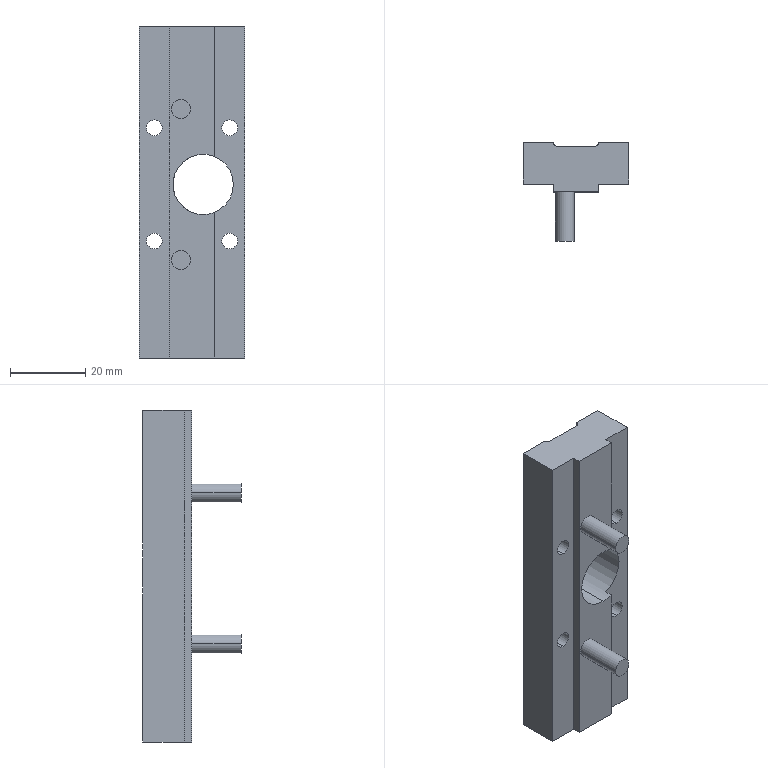Part | SolidWorks | features BaseBody 1 | 1 solid | 33 faces | box 28 x 26.1 x 88 mm | volume 25740 mm3 | cylinder 17 | plane 16 | commonest cylinder face diameters 4.2 x8 5 x4 2 x3 16 x2
STEP:
#1=CARTESIAN_POINT('',(-10.,2.,28.9));
#2=VERTEX_POINT('',#1);
#3=CARTESIAN_POINT('',(-10.,2.,33.1));
#4=VERTEX_POINT('',#3);
#5=CARTESIAN_POINT('',(-10.,2.,31.));
#6=DIRECTION('',(0.,1.,0.));
#7=DIRECTION('',(0.,0.,1.));
#8=AXIS2_PLACEMENT_3D('',#5,#6,#7);
#9=CIRCLE('',#8,2.1);
#10=EDGE_CURVE('',#2,#4,#9,.T.);
#11=ORIENTED_EDGE('',*,*,#10,.F.);
#12=CARTESIAN_POINT('',(-10.,13.,28.9));
#13=VERTEX_POINT('',#12);
#14=CARTESIAN_POINT('',(-10.,13.,28.9));
#15=DIRECTION('',(0.,1.,0.));
#16=VECTOR('',#15,1000.);
#17=LINE('',#14,#16);
#18=EDGE_CURVE('',#2,#13,#17,.T.);
#19=ORIENTED_EDGE('',*,*,#18,.T.);
#20=CARTESIAN_POINT('',(-10.,13.,33.1));
#21=VERTEX_POINT('',#20);
#22=CARTESIAN_POINT('',(-10.,13.,31.));
#23=DIRECTION('',(0.,1.,0.));
#24=DIRECTION('',(0.,0.,1.));
#25=AXIS2_PLACEMENT_3D('',#22,#23,#24);
#26=CIRCLE('',#25,2.1);
#27=EDGE_CURVE('',#13,#21,#26,.T.);
#28=ORIENTED_EDGE('',*,*,#27,.T.);
#29=CARTESIAN_POINT('',(-10.,13.,33.1));
#30=DIRECTION('',(0.,1.,0.));
#31=VECTOR('',#30,1000.);
#32=LINE('',#29,#31);
#33=EDGE_CURVE('',#4,#21,#32,.T.);
#34=ORIENTED_EDGE('',*,*,#33,.F.);
#35=EDGE_LOOP('',(#11,#19,#28,#34));
#36=FACE_OUTER_BOUND('',#35,.T.);
#37=CARTESIAN_POINT('',(-10.,13.,31.));
#38=DIRECTION('',(0.,1.,0.));
#39=DIRECTION('',(0.,0.,1.));
#40=AXIS2_PLACEMENT_3D('',#37,#38,#39);
#41=CYLINDRICAL_SURFACE('',#40,2.1);
#42=ADVANCED_FACE('',(#36),#41,.F.);
#43=CARTESIAN_POINT('',(-10.,2.,58.9));
#44=VERTEX_POINT('',#43);
#45=CARTESIAN_POINT('',(-10.,2.,63.1));
#46=VERTEX_POINT('',#45);
#47=CARTESIAN_POINT('',(-10.,2.,61.));
#48=DIRECTION('',(0.,1.,0.));
#49=DIRECTION('',(0.,0.,1.));
#50=AXIS2_PLACEMENT_3D('',#47,#48,#49);
#51=CIRCLE('',#50,2.1);
#52=EDGE_CURVE('',#44,#46,#51,.T.);
#53=ORIENTED_EDGE('',*,*,#52,.F.);
#54=CARTESIAN_POINT('',(-10.,13.,58.9));
#55=VERTEX_POINT('',#54);
#56=CARTESIAN_POINT('',(-10.,13.,58.9));
#57=DIRECTION('',(0.,1.,0.));
#58=VECTOR('',#57,1000.);
#59=LINE('',#56,#58);
#60=EDGE_CURVE('',#44,#55,#59,.T.);
#61=ORIENTED_EDGE('',*,*,#60,.T.);
#62=CARTESIAN_POINT('',(-10.,13.,63.1));
#63=VERTEX_POINT('',#62);
#64=CARTESIAN_POINT('',(-10.,13.,61.));
#65=DIRECTION('',(0.,1.,0.));
#66=DIRECTION('',(0.,0.,1.));
#67=AXIS2_PLACEMENT_3D('',#64,#65,#66);
#68=CIRCLE('',#67,2.1);
#69=EDGE_CURVE('',#55,#63,#68,.T.);
#70=ORIENTED_EDGE('',*,*,#69,.T.);
#71=CARTESIAN_POINT('',(-10.,13.,63.1));
#72=DIRECTION('',(0.,1.,0.));
#73=VECTOR('',#72,1000.);
#74=LINE('',#71,#73);
#75=EDGE_CURVE('',#46,#63,#74,.T.);
#76=ORIENTED_EDGE('',*,*,#75,.F.);
#77=EDGE_LOOP('',(#53,#61,#70,#76));
#78=FACE_OUTER_BOUND('',#77,.T.);
#79=CARTESIAN_POINT('',(-10.,13.,61.));
#80=DIRECTION('',(0.,1.,0.));
#81=DIRECTION('',(0.,0.,1.));
#82=AXIS2_PLACEMENT_3D('',#79,#80,#81);
#83=CYLINDRICAL_SURFACE('',#82,2.1);
#84=ADVANCED_FACE('',(#78),#83,.F.);
#85=CARTESIAN_POINT('',(10.,2.,28.9));
#86=VERTEX_POINT('',#85);
#87=CARTESIAN_POINT('',(10.,2.,33.1));
#88=VERTEX_POINT('',#87);
#89=CARTESIAN_POINT('',(10.,2.,31.));
#90=DIRECTION('',(0.,1.,0.));
#91=DIRECTION('',(-1.,0.,0.));
#92=AXIS2_PLACEMENT_3D('',#89,#90,#91);
#93=CIRCLE('',#92,2.1);
#94=EDGE_CURVE('',#86,#88,#93,.T.);
#95=ORIENTED_EDGE('',*,*,#94,.F.);
#96=CARTESIAN_POINT('',(10.,13.,28.9));
#97=VERTEX_POINT('',#96);
#98=CARTESIAN_POINT('',(10.,13.,28.9));
#99=DIRECTION('',(0.,1.,0.));
#100=VECTOR('',#99,1000.);
#101=LINE('',#98,#100);
#102=EDGE_CURVE('',#86,#97,#101,.T.);
#103=ORIENTED_EDGE('',*,*,#102,.T.);
#104=CARTESIAN_POINT('',(10.,13.,33.1));
#105=VERTEX_POINT('',#104);
#106=CARTESIAN_POINT('',(10.,13.,31.));
#107=DIRECTION('',(0.,1.,0.));
#108=DIRECTION('',(0.,0.,1.));
#109=AXIS2_PLACEMENT_3D('',#106,#107,#108);
#110=CIRCLE('',#109,2.1);
#111=EDGE_CURVE('',#97,#105,#110,.T.);
#112=ORIENTED_EDGE('',*,*,#111,.T.);
#113=CARTESIAN_POINT('',(10.,13.,33.1));
#114=DIRECTION('',(0.,1.,0.));
#115=VECTOR('',#114,1000.);
#116=LINE('',#113,#115);
#117=EDGE_CURVE('',#88,#105,#116,.T.);
#118=ORIENTED_EDGE('',*,*,#117,.F.);
#119=EDGE_LOOP('',(#95,#103,#112,#118));
#120=FACE_OUTER_BOUND('',#119,.T.);
#121=CARTESIAN_POINT('',(10.,13.,31.));
#122=DIRECTION('',(0.,1.,0.));
#123=DIRECTION('',(0.,0.,1.));
#124=AXIS2_PLACEMENT_3D('',#121,#122,#123);
#125=CYLINDRICAL_SURFACE('',#124,2.1);
#126=ADVANCED_FACE('',(#120),#125,.F.);
#127=CARTESIAN_POINT('',(10.,2.,58.9));
#128=VERTEX_POINT('',#127);
#129=CARTESIAN_POINT('',(10.,2.,63.1));
#130=VERTEX_POINT('',#129);
#131=CARTESIAN_POINT('',(10.,2.,61.));
#132=DIRECTION('',(0.,1.,0.));
#133=DIRECTION('',(-1.,0.,0.));
#134=AXIS2_PLACEMENT_3D('',#131,#132,#133);
#135=CIRCLE('',#134,2.1);
#136=EDGE_CURVE('',#128,#130,#135,.T.);
#137=ORIENTED_EDGE('',*,*,#136,.F.);
#138=CARTESIAN_POINT('',(10.,13.,58.9));
#139=VERTEX_POINT('',#138);
#140=CARTESIAN_POINT('',(10.,13.,58.9));
#141=DIRECTION('',(0.,1.,0.));
#142=VECTOR('',#141,1000.);
#143=LINE('',#140,#142);
#144=EDGE_CURVE('',#128,#139,#143,.T.);
#145=ORIENTED_EDGE('',*,*,#144,.T.);
#146=CARTESIAN_POINT('',(10.,13.,63.1));
#147=VERTEX_POINT('',#146);
#148=CARTESIAN_POINT('',(10.,13.,61.));
#149=DIRECTION('',(0.,1.,0.));
#150=DIRECTION('',(0.,0.,1.));
#151=AXIS2_PLACEMENT_3D('',#148,#149,#150);
#152=CIRCLE('',#151,2.1);
#153=EDGE_CURVE('',#139,#147,#152,.T.);
#154=ORIENTED_EDGE('',*,*,#153,.T.);
#155=CARTESIAN_POINT('',(10.,13.,63.1));
#156=DIRECTION('',(0.,1.,0.));
#157=VECTOR('',#156,1000.);
#158=LINE('',#155,#157);
#159=EDGE_CURVE('',#130,#147,#158,.T.);
#160=ORIENTED_EDGE('',*,*,#159,.F.);
#161=EDGE_LOOP('',(#137,#145,#154,#160));
#162=FACE_OUTER_BOUND('',#161,.T.);
#163=CARTESIAN_POINT('',(10.,13.,61.));
#164=DIRECTION('',(0.,1.,0.));
#165=DIRECTION('',(0.,0.,1.));
#166=AXIS2_PLACEMENT_3D('',#163,#164,#165);
#167=CYLINDRICAL_SURFACE('',#166,2.1);
#168=ADVANCED_FACE('',(#162),#167,.F.);
#169=CARTESIAN_POINT('',(2.95,12.,54.));
#170=VERTEX_POINT('',#169);
#171=CARTESIAN_POINT('',(-5.,12.,46.893));
#172=VERTEX_POINT('',#171);
#173=CARTESIAN_POINT('',(2.95,12.,46.));
#174=DIRECTION('',(0.,-1.,0.));
#175=DIRECTION('',(1.,0.,0.));
#176=AXIS2_PLACEMENT_3D('',#173,#174,#175);
#177=CIRCLE('',#176,8.);
#178=EDGE_CURVE('',#170,#172,#177,.T.);
#179=ORIENTED_EDGE('',*,*,#178,.F.);
#180=CARTESIAN_POINT('',(2.95,0.,54.));
#181=VERTEX_POINT('',#180);
#182=CARTESIAN_POINT('',(2.95,0.,54.));
#183=DIRECTION('',(0.,-1.,0.));
#184=VECTOR('',#183,1000.);
#185=LINE('',#182,#184);
#186=EDGE_CURVE('',#170,#181,#185,.T.);
#187=ORIENTED_EDGE('',*,*,#186,.T.);
#188=CARTESIAN_POINT('',(2.95,0.,38.));
#189=VERTEX_POINT('',#188);
#190=CARTESIAN_POINT('',(2.95,0.,46.));
#191=DIRECTION('',(0.,-1.,0.));
#192=DIRECTION('',(0.,0.,-1.));
#193=AXIS2_PLACEMENT_3D('',#190,#191,#192);
#194=CIRCLE('',#193,8.);
#195=EDGE_CURVE('',#181,#189,#194,.T.);
#196=ORIENTED_EDGE('',*,*,#195,.T.);
#197=CARTESIAN_POINT('',(2.95,12.,38.));
#198=VERTEX_POINT('',#197);
#199=CARTESIAN_POINT('',(2.95,0.,38.));
#200=DIRECTION('',(0.,-1.,0.));
#201=VECTOR('',#200,1000.);
#202=LINE('',#199,#201);
#203=EDGE_CURVE('',#198,#189,#202,.T.);
#204=ORIENTED_EDGE('',*,*,#203,.F.);
#205=CARTESIAN_POINT('',(-5.,12.,45.107));
#206=VERTEX_POINT('',#205);
#207=CARTESIAN_POINT('',(2.95,12.,46.));
#208=DIRECTION('',(0.,-1.,0.));
#209=DIRECTION('',(1.,0.,0.));
#210=AXIS2_PLACEMENT_3D('',#207,#208,#209);
#211=CIRCLE('',#210,8.);
#212=EDGE_CURVE('',#206,#198,#211,.T.);
#213=ORIENTED_EDGE('',*,*,#212,.F.);
#214=CARTESIAN_POINT('',(-5.,12.,46.893));
#215=CARTESIAN_POINT('',(-5.033,12.,46.595));
#216=CARTESIAN_POINT('',(-5.067,12.003,46.));
#217=CARTESIAN_POINT('',(-5.033,12.,45.405));
#218=CARTESIAN_POINT('',(-5.,12.,45.107));
#219=B_SPLINE_CURVE_WITH_KNOTS('',3,(#214,#215,#216,#217,#218),.UNSPECIFIED.,.F.,.F.,(4,1,4),(0.,0.5,1.),.UNSPECIFIED.);
#220=EDGE_CURVE('',#172,#206,#219,.T.);
#221=ORIENTED_EDGE('',*,*,#220,.F.);
#222=EDGE_LOOP('',(#179,#187,#196,#204,#213,#221));
#223=FACE_OUTER_BOUND('',#222,.T.);
#224=CARTESIAN_POINT('',(2.95,0.,46.));
#225=DIRECTION('',(0.,-1.,0.));
#226=DIRECTION('',(0.,0.,-1.));
#227=AXIS2_PLACEMENT_3D('',#224,#225,#226);
#228=CYLINDRICAL_SURFACE('',#227,8.);
#229=ADVANCED_FACE('',(#223),#228,.F.);
#230=CARTESIAN_POINT('',(-5.45,-13.1,66.));
#231=VERTEX_POINT('',#230);
#232=CARTESIAN_POINT('',(-0.45,-13.1,66.));
#233=VERTEX_POINT('',#232);
#234=CARTESIAN_POINT('',(-2.95,-13.1,66.));
#235=DIRECTION('',(0.,1.,0.));
#236=DIRECTION('',(-1.,0.,0.));
#237=AXIS2_PLACEMENT_3D('',#234,#235,#236);
#238=CIRCLE('',#237,2.5);
#239=EDGE_CURVE('',#231,#233,#238,.T.);
#240=ORIENTED_EDGE('',*,*,#239,.T.);
#241=CARTESIAN_POINT('',(-0.45,0.,66.));
#242=VERTEX_POINT('',#241);
#243=CARTESIAN_POINT('',(-0.45,-13.1,66.));
#244=DIRECTION('',(0.,1.,0.));
#245=VECTOR('',#244,1000.);
#246=LINE('',#243,#245);
#247=EDGE_CURVE('',#233,#242,#246,.T.);
#248=ORIENTED_EDGE('',*,*,#247,.T.);
#249=CARTESIAN_POINT('',(-5.45,0.,66.));
#250=VERTEX_POINT('',#249);
#251=CARTESIAN_POINT('',(-2.95,0.,66.));
#252=DIRECTION('',(0.,-1.,0.));
#253=DIRECTION('',(1.,0.,0.));
#254=AXIS2_PLACEMENT_3D('',#251,#252,#253);
#255=CIRCLE('',#254,2.5);
#256=EDGE_CURVE('',#242,#250,#255,.T.);
#257=ORIENTED_EDGE('',*,*,#256,.T.);
#258=CARTESIAN_POINT('',(-5.45,-13.1,66.));
#259=DIRECTION('',(0.,1.,0.));
#260=VECTOR('',#259,1000.);
#261=LINE('',#258,#260);
#262=EDGE_CURVE('',#231,#250,#261,.T.);
#263=ORIENTED_EDGE('',*,*,#262,.F.);
#264=EDGE_LOOP('',(#240,#248,#257,#263));
#265=FACE_OUTER_BOUND('',#264,.T.);
#266=CARTESIAN_POINT('',(-2.95,-13.1,66.));
#267=DIRECTION('',(0.,1.,0.));
#268=DIRECTION('',(-1.,0.,0.));
#269=AXIS2_PLACEMENT_3D('',#266,#267,#268);
#270=CYLINDRICAL_SURFACE('',#269,2.5);
#271=ADVANCED_FACE('',(#265),#270,.T.);
#272=CARTESIAN_POINT('',(-5.45,-13.1,26.));
#273=VERTEX_POINT('',#272);
#274=CARTESIAN_POINT('',(-0.45,-13.1,26.));
#275=VERTEX_POINT('',#274);
#276=CARTESIAN_POINT('',(-2.95,-13.1,26.));
#277=DIRECTION('',(0.,1.,0.));
#278=DIRECTION('',(-1.,0.,0.));
#279=AXIS2_PLACEMENT_3D('',#276,#277,#278);
#280=CIRCLE('',#279,2.5);
#281=EDGE_CURVE('',#273,#275,#280,.T.);
#282=ORIENTED_EDGE('',*,*,#281,.T.);
#283=CARTESIAN_POINT('',(-0.45,0.,26.));
#284=VERTEX_POINT('',#283);
#285=CARTESIAN_POINT('',(-0.45,-13.1,26.));
#286=DIRECTION('',(0.,1.,0.));
#287=VECTOR('',#286,1000.);
#288=LINE('',#285,#287);
#289=EDGE_CURVE('',#275,#284,#288,.T.);
#290=ORIENTED_EDGE('',*,*,#289,.T.);
#291=CARTESIAN_POINT('',(-5.45,0.,26.));
#292=VERTEX_POINT('',#291);
#293=CARTESIAN_POINT('',(-2.95,0.,26.));
#294=DIRECTION('',(0.,-1.,0.));
#295=DIRECTION('',(1.,0.,0.));
#296=AXIS2_PLACEMENT_3D('',#293,#294,#295);
#297=CIRCLE('',#296,2.5);
#298=EDGE_CURVE('',#284,#292,#297,.T.);
#299=ORIENTED_EDGE('',*,*,#298,.T.);
#300=CARTESIAN_POINT('',(-5.45,-13.1,26.));
#301=DIRECTION('',(0.,1.,0.));
#302=VECTOR('',#301,1000.);
#303=LINE('',#300,#302);
#304=EDGE_CURVE('',#273,#292,#303,.T.);
#305=ORIENTED_EDGE('',*,*,#304,.F.);
#306=EDGE_LOOP('',(#282,#290,#299,#305));
#307=FACE_OUTER_BOUND('',#306,.T.);
#308=CARTESIAN_POINT('',(-2.95,-13.1,26.));
#309=DIRECTION('',(0.,1.,0.));
#310=DIRECTION('',(-1.,0.,0.));
#311=AXIS2_PLACEMENT_3D('',#308,#309,#310);
#312=CYLINDRICAL_SURFACE('',#311,2.5);
#313=ADVANCED_FACE('',(#307),#312,.T.);
#314=CARTESIAN_POINT('',(5.,12.,53.733));
#315=VERTEX_POINT('',#314);
#316=CARTESIAN_POINT('',(5.,12.,88.));
#317=VERTEX_POINT('',#316);
#318=CARTESIAN_POINT('',(5.,12.,0.));
#319=DIRECTION('',(0.,0.,1.));
#320=VECTOR('',#319,1000.);
#321=LINE('',#318,#320);
#322=EDGE_CURVE('',#315,#317,#321,.T.);
#323=ORIENTED_EDGE('',*,*,#322,.F.);
#324=CARTESIAN_POINT('',(2.95,12.,46.));
#325=DIRECTION('',(0.,-1.,0.));
#326=DIRECTION('',(1.,0.,0.));
#327=AXIS2_PLACEMENT_3D('',#324,#325,#326);
#328=CIRCLE('',#327,8.);
#329=EDGE_CURVE('',#315,#170,#328,.T.);
#330=ORIENTED_EDGE('',*,*,#329,.T.);
#331=ORIENTED_EDGE('',*,*,#178,.T.);
#332=CARTESIAN_POINT('',(-5.,12.,88.));
#333=VERTEX_POINT('',#332);
#334=CARTESIAN_POINT('',(-5.,12.,0.));
#335=DIRECTION('',(0.,0.,1.));
#336=VECTOR('',#335,1000.);
#337=LINE('',#334,#336);
#338=EDGE_CURVE('',#172,#333,#337,.T.);
#339=ORIENTED_EDGE('',*,*,#338,.T.);
#340=CARTESIAN_POINT('',(14.,12.,88.));
#341=DIRECTION('',(1.,0.,0.));
#342=VECTOR('',#341,1000.);
#343=LINE('',#340,#342);
#344=EDGE_CURVE('',#333,#317,#343,.T.);
#345=ORIENTED_EDGE('',*,*,#344,.T.);
#346=EDGE_LOOP('',(#323,#330,#331,#339,#345));
#347=FACE_OUTER_BOUND('',#346,.T.);
#348=CARTESIAN_POINT('',(-5.,12.,0.));
#349=DIRECTION('',(0.,-1.,0.));
#350=DIRECTION('',(0.,0.,-1.));
#351=AXIS2_PLACEMENT_3D('',#348,#349,#350);
#352=PLANE('',#351);
#353=ADVANCED_FACE('',(#347),#352,.F.);
#354=CARTESIAN_POINT('',(6.,2.,0.));
#355=VERTEX_POINT('',#354);
#356=CARTESIAN_POINT('',(6.,2.,38.604));
#357=VERTEX_POINT('',#356);
#358=CARTESIAN_POINT('',(6.,2.,0.));
#359=DIRECTION('',(0.,0.,1.));
#360=VECTOR('',#359,1000.);
#361=LINE('',#358,#360);
#362=EDGE_CURVE('',#355,#357,#361,.T.);
#363=ORIENTED_EDGE('',*,*,#362,.T.);
#364=CARTESIAN_POINT('',(6.,0.,38.604));
#365=VERTEX_POINT('',#364);
#366=CARTESIAN_POINT('',(6.,0.,38.604));
#367=DIRECTION('',(0.,-1.,0.));
#368=VECTOR('',#367,1000.);
#369=LINE('',#366,#368);
#370=EDGE_CURVE('',#357,#365,#369,.T.);
#371=ORIENTED_EDGE('',*,*,#370,.T.);
#372=CARTESIAN_POINT('',(6.,0.,0.));
#373=VERTEX_POINT('',#372);
#374=CARTESIAN_POINT('',(6.,0.,0.));
#375=DIRECTION('',(0.,0.,1.));
#376=VECTOR('',#375,1000.);
#377=LINE('',#374,#376);
#378=EDGE_CURVE('',#373,#365,#377,.T.);
#379=ORIENTED_EDGE('',*,*,#378,.F.);
#380=CARTESIAN_POINT('',(6.,2.,0.));
#381=DIRECTION('',(0.,-1.,0.));
#382=VECTOR('',#381,1000.);
#383=LINE('',#380,#382);
#384=EDGE_CURVE('',#355,#373,#383,.T.);
#385=ORIENTED_EDGE('',*,*,#384,.F.);
#386=EDGE_LOOP('',(#363,#371,#379,#385));
#387=FACE_OUTER_BOUND('',#386,.T.);
#388=CARTESIAN_POINT('',(6.,2.,0.));
#389=DIRECTION('',(-1.,0.,0.));
#390=DIRECTION('',(0.,0.,1.));
#391=AXIS2_PLACEMENT_3D('',#388,#389,#390);
#392=PLANE('',#391);
#393=ADVANCED_FACE('',(#387),#392,.F.);
#394=CARTESIAN_POINT('',(6.,13.,53.396));
#395=VERTEX_POINT('',#394);
#396=CARTESIAN_POINT('',(6.,13.,88.));
#397=VERTEX_POINT('',#396);
#398=CARTESIAN_POINT('',(6.,13.,0.));
#399=DIRECTION('',(0.,0.,1.));
#400=VECTOR('',#399,1000.);
#401=LINE('',#398,#400);
#402=EDGE_CURVE('',#395,#397,#401,.T.);
#403=ORIENTED_EDGE('',*,*,#402,.F.);
#404=CARTESIAN_POINT('',(6.,13.,53.396));
#405=CARTESIAN_POINT('',(6.,12.935,53.396));
#406=CARTESIAN_POINT('',(5.994,12.869,53.398));
#407=CARTESIAN_POINT('',(5.974,12.771,53.407));
#408=CARTESIAN_POINT('',(5.966,12.738,53.41));
#409=CARTESIAN_POINT('',(5.951,12.689,53.416));
#410=CARTESIAN_POINT('',(5.943,12.665,53.419));
#411=CARTESIAN_POINT('',(5.933,12.641,53.423));
#412=CARTESIAN_POINT('',(5.927,12.625,53.425));
#413=CARTESIAN_POINT('',(5.923,12.616,53.427));
#414=CARTESIAN_POINT('',(5.898,12.555,53.437));
#415=CARTESIAN_POINT('',(5.868,12.5,53.449));
#416=CARTESIAN_POINT('',(5.814,12.418,53.47));
#417=CARTESIAN_POINT('',(5.794,12.391,53.478));
#418=CARTESIAN_POINT('',(5.761,12.351,53.49));
#419=CARTESIAN_POINT('',(5.744,12.331,53.496));
#420=CARTESIAN_POINT('',(5.722,12.308,53.504));
#421=CARTESIAN_POINT('',(5.713,12.299,53.508));
#422=CARTESIAN_POINT('',(5.707,12.292,53.51));
#423=CARTESIAN_POINT('',(5.702,12.288,53.512));
#424=CARTESIAN_POINT('',(5.67,12.257,53.523));
#425=CARTESIAN_POINT('',(5.631,12.221,53.538));
#426=CARTESIAN_POINT('',(5.552,12.165,53.565));
#427=CARTESIAN_POINT('',(5.522,12.146,53.576));
#428=CARTESIAN_POINT('',(5.456,12.109,53.598));
#429=CARTESIAN_POINT('',(5.417,12.09,53.61));
#430=CARTESIAN_POINT('',(5.224,12.011,53.672));
#431=CARTESIAN_POINT('',(5.091,12.,53.709));
#432=CARTESIAN_POINT('',(5.,12.,53.733));
#433=B_SPLINE_CURVE_WITH_KNOTS('',3,(#404,#405,#406,#407,#408,#409,#410,#411,#412,#413,#414,#415,#416,#417,#418,#419,#420,#421,#422,#423,#424,#425,#426,#427,#428,#429,#430,#431,#432),.UNSPECIFIED.,.F.,.F.,(4,2,2,1,2,2,2,2,1,1,2,2,2,2,2,4),(0.,0.125,0.1875,0.2188,0.2344,0.25,0.375,0.4375,0.4688,0.4844,0.4922,0.5,0.625,0.6875,0.75,1.),.UNSPECIFIED.);
#434=EDGE_CURVE('',#395,#315,#433,.T.);
#435=ORIENTED_EDGE('',*,*,#434,.T.);
#436=ORIENTED_EDGE('',*,*,#322,.T.);
#437=CARTESIAN_POINT('',(5.,13.,88.));
#438=DIRECTION('',(0.,0.,1.));
#439=DIRECTION('',(1.,0.,0.));
#440=AXIS2_PLACEMENT_3D('',#437,#438,#439);
#441=CIRCLE('',#440,1.);
#442=EDGE_CURVE('',#317,#397,#441,.T.);
#443=ORIENTED_EDGE('',*,*,#442,.T.);
#444=EDGE_LOOP('',(#403,#435,#436,#443));
#445=FACE_OUTER_BOUND('',#444,.T.);
#446=CARTESIAN_POINT('',(5.,13.,0.));
#447=DIRECTION('',(0.,0.,1.));
#448=DIRECTION('',(1.,0.,0.));
#449=AXIS2_PLACEMENT_3D('',#446,#447,#448);
#450=CYLINDRICAL_SURFACE('',#449,1.);
#451=ADVANCED_FACE('',(#445),#450,.F.);
#452=CARTESIAN_POINT('',(10.,13.,31.));
#453=DIRECTION('',(0.,1.,0.));
#454=DIRECTION('',(0.,0.,1.));
#455=AXIS2_PLACEMENT_3D('',#452,#453,#454);
#456=CIRCLE('',#455,2.1);
#457=EDGE_CURVE('',#105,#97,#456,.T.);
#458=ORIENTED_EDGE('',*,*,#457,.F.);
#459=ORIENTED_EDGE('',*,*,#111,.F.);
#460=EDGE_LOOP('',(#458,#459));
#461=FACE_BOUND('',#460,.T.);
#462=CARTESIAN_POINT('',(10.,13.,61.));
#463=DIRECTION('',(0.,1.,0.));
#464=DIRECTION('',(0.,0.,1.));
#465=AXIS2_PLACEMENT_3D('',#462,#463,#464);
#466=CIRCLE('',#465,2.1);
#467=EDGE_CURVE('',#147,#139,#466,.T.);
#468=ORIENTED_EDGE('',*,*,#467,.F.);
#469=ORIENTED_EDGE('',*,*,#153,.F.);
#470=EDGE_LOOP('',(#468,#469));
#471=FACE_BOUND('',#470,.T.);
#472=CARTESIAN_POINT('',(6.,13.,0.));
#473=VERTEX_POINT('',#472);
#474=CARTESIAN_POINT('',(6.,13.,38.604));
#475=VERTEX_POINT('',#474);
#476=CARTESIAN_POINT('',(6.,13.,0.));
#477=DIRECTION('',(0.,0.,1.));
#478=VECTOR('',#477,1000.);
#479=LINE('',#476,#478);
#480=EDGE_CURVE('',#473,#475,#479,.T.);
#481=ORIENTED_EDGE('',*,*,#480,.T.);
#482=CARTESIAN_POINT('',(2.95,13.,46.));
#483=DIRECTION('',(0.,-1.,0.));
#484=DIRECTION('',(0.,0.,-1.));
#485=AXIS2_PLACEMENT_3D('',#482,#483,#484);
#486=CIRCLE('',#485,8.);
#487=EDGE_CURVE('',#475,#395,#486,.T.);
#488=ORIENTED_EDGE('',*,*,#487,.T.);
#489=ORIENTED_EDGE('',*,*,#402,.T.);
#490=CARTESIAN_POINT('',(14.,13.,88.));
#491=VERTEX_POINT('',#490);
#492=CARTESIAN_POINT('',(0.,13.,88.));
#493=DIRECTION('',(-1.,0.,0.));
#494=VECTOR('',#493,1000.);
#495=LINE('',#492,#494);
#496=EDGE_CURVE('',#491,#397,#495,.T.);
#497=ORIENTED_EDGE('',*,*,#496,.F.);
#498=CARTESIAN_POINT('',(14.,13.,0.));
#499=VERTEX_POINT('',#498);
#500=CARTESIAN_POINT('',(14.,13.,0.));
#501=DIRECTION('',(0.,0.,1.));
#502=VECTOR('',#501,1000.);
#503=LINE('',#500,#502);
#504=EDGE_CURVE('',#499,#491,#503,.T.);
#505=ORIENTED_EDGE('',*,*,#504,.F.);
#506=CARTESIAN_POINT('',(-14.,13.,0.));
#507=DIRECTION('',(1.,0.,0.));
#508=VECTOR('',#507,1000.);
#509=LINE('',#506,#508);
#510=EDGE_CURVE('',#473,#499,#509,.T.);
#511=ORIENTED_EDGE('',*,*,#510,.F.);
#512=EDGE_LOOP('',(#481,#488,#489,#497,#505,#511));
#513=FACE_OUTER_BOUND('',#512,.T.);
#514=CARTESIAN_POINT('',(0.,13.,0.));
#515=DIRECTION('',(0.,-1.,0.));
#516=DIRECTION('',(-1.,0.,0.));
#517=AXIS2_PLACEMENT_3D('',#514,#515,#516);
#518=PLANE('',#517);
#519=ADVANCED_FACE('',(#461,#471,#513),#518,.F.);
#520=CARTESIAN_POINT('',(-14.,2.,0.));
#521=VERTEX_POINT('',#520);
#522=CARTESIAN_POINT('',(-14.,2.,88.));
#523=VERTEX_POINT('',#522);
#524=CARTESIAN_POINT('',(-14.,2.,0.));
#525=DIRECTION('',(0.,0.,1.));
#526=VECTOR('',#525,1000.);
#527=LINE('',#524,#526);
#528=EDGE_CURVE('',#521,#523,#527,.T.);
#529=ORIENTED_EDGE('',*,*,#528,.T.);
#530=CARTESIAN_POINT('',(-14.,13.,88.));
#531=VERTEX_POINT('',#530);
#532=CARTESIAN_POINT('',(-14.,13.,88.));
#533=DIRECTION('',(0.,-1.,0.));
#534=VECTOR('',#533,1000.);
#535=LINE('',#532,#534);
#536=EDGE_CURVE('',#531,#523,#535,.T.);
#537=ORIENTED_EDGE('',*,*,#536,.F.);
#538=CARTESIAN_POINT('',(-14.,13.,0.));
#539=VERTEX_POINT('',#538);
#540=CARTESIAN_POINT('',(-14.,13.,60.));
#541=DIRECTION('',(0.,0.,-1.));
#542=VECTOR('',#541,1000.);
#543=LINE('',#540,#542);
#544=EDGE_CURVE('',#531,#539,#543,.T.);
#545=ORIENTED_EDGE('',*,*,#544,.T.);
#546=CARTESIAN_POINT('',(-14.,13.,0.));
#547=DIRECTION('',(0.,-1.,0.));
#548=VECTOR('',#547,1000.);
#549=LINE('',#546,#548);
#550=EDGE_CURVE('',#539,#521,#549,.T.);
#551=ORIENTED_EDGE('',*,*,#550,.T.);
#552=EDGE_LOOP('',(#529,#537,#545,#551));
#553=FACE_OUTER_BOUND('',#552,.T.);
#554=CARTESIAN_POINT('',(-14.,13.,60.));
#555=DIRECTION('',(-1.,0.,0.));
#556=DIRECTION('',(0.,0.,1.));
#557=AXIS2_PLACEMENT_3D('',#554,#555,#556);
#558=PLANE('',#557);
#559=ADVANCED_FACE('',(#553),#558,.T.);
#560=ORIENTED_EDGE('',*,*,#442,.F.);
#561=ORIENTED_EDGE('',*,*,#344,.F.);
#562=CARTESIAN_POINT('',(-6.,13.,88.));
#563=VERTEX_POINT('',#562);
#564=CARTESIAN_POINT('',(-5.,13.,88.));
#565=DIRECTION('',(0.,0.,1.));
#566=DIRECTION('',(1.,0.,0.));
#567=AXIS2_PLACEMENT_3D('',#564,#565,#566);
#568=CIRCLE('',#567,1.);
#569=EDGE_CURVE('',#563,#333,#568,.T.);
#570=ORIENTED_EDGE('',*,*,#569,.F.);
#571=CARTESIAN_POINT('',(0.,13.,88.));
#572=DIRECTION('',(-1.,0.,0.));
#573=VECTOR('',#572,1000.);
#574=LINE('',#571,#573);
#575=EDGE_CURVE('',#563,#531,#574,.T.);
#576=ORIENTED_EDGE('',*,*,#575,.T.);
#577=ORIENTED_EDGE('',*,*,#536,.T.);
#578=CARTESIAN_POINT('',(-6.,2.,88.));
#579=VERTEX_POINT('',#578);
#580=CARTESIAN_POINT('',(14.,2.,88.));
#581=DIRECTION('',(-1.,0.,0.));
#582=VECTOR('',#581,1000.);
#583=LINE('',#580,#582);
#584=EDGE_CURVE('',#579,#523,#583,.T.);
#585=ORIENTED_EDGE('',*,*,#584,.F.);
#586=CARTESIAN_POINT('',(-6.,0.,88.));
#587=VERTEX_POINT('',#586);
#588=CARTESIAN_POINT('',(-6.,13.,88.));
#589=DIRECTION('',(0.,1.,0.));
#590=VECTOR('',#589,1000.);
#591=LINE('',#588,#590);
#592=EDGE_CURVE('',#587,#579,#591,.T.);
#593=ORIENTED_EDGE('',*,*,#592,.F.);
#594=CARTESIAN_POINT('',(6.,0.,88.));
#595=VERTEX_POINT('',#594);
#596=CARTESIAN_POINT('',(0.,0.,88.));
#597=DIRECTION('',(-1.,0.,0.));
#598=VECTOR('',#597,1000.);
#599=LINE('',#596,#598);
#600=EDGE_CURVE('',#595,#587,#599,.T.);
#601=ORIENTED_EDGE('',*,*,#600,.F.);
#602=CARTESIAN_POINT('',(6.,2.,88.));
#603=VERTEX_POINT('',#602);
#604=CARTESIAN_POINT('',(6.,13.,88.));
#605=DIRECTION('',(0.,-1.,0.));
#606=VECTOR('',#605,1000.);
#607=LINE('',#604,#606);
#608=EDGE_CURVE('',#603,#595,#607,.T.);
#609=ORIENTED_EDGE('',*,*,#608,.F.);
#610=CARTESIAN_POINT('',(14.,2.,88.));
#611=VERTEX_POINT('',#610);
#612=CARTESIAN_POINT('',(14.,2.,88.));
#613=DIRECTION('',(-1.,0.,0.));
#614=VECTOR('',#613,1000.);
#615=LINE('',#612,#614);
#616=EDGE_CURVE('',#611,#603,#615,.T.);
#617=ORIENTED_EDGE('',*,*,#616,.F.);
#618=CARTESIAN_POINT('',(14.,13.,88.));
#619=DIRECTION('',(0.,-1.,0.));
#620=VECTOR('',#619,1000.);
#621=LINE('',#618,#620);
#622=EDGE_CURVE('',#491,#611,#621,.T.);
#623=ORIENTED_EDGE('',*,*,#622,.F.);
#624=ORIENTED_EDGE('',*,*,#496,.T.);
#625=EDGE_LOOP('',(#560,#561,#570,#576,#577,#585,#593,#601,#609,#617,#623,#624));
#626=FACE_OUTER_BOUND('',#625,.T.);
#627=CARTESIAN_POINT('',(14.,13.,88.));
#628=DIRECTION('',(0.,0.,1.));
#629=DIRECTION('',(1.,0.,0.));
#630=AXIS2_PLACEMENT_3D('',#627,#628,#629);
#631=PLANE('',#630);
#632=ADVANCED_FACE('',(#626),#631,.T.);
#633=CARTESIAN_POINT('',(14.,2.,0.));
#634=VERTEX_POINT('',#633);
#635=CARTESIAN_POINT('',(14.,2.,0.));
#636=DIRECTION('',(0.,0.,1.));
#637=VECTOR('',#636,1000.);
#638=LINE('',#635,#637);
#639=EDGE_CURVE('',#634,#611,#638,.T.);
#640=ORIENTED_EDGE('',*,*,#639,.F.);
#641=CARTESIAN_POINT('',(14.,13.,0.));
#642=DIRECTION('',(0.,-1.,0.));
#643=VECTOR('',#642,1000.);
#644=LINE('',#641,#643);
#645=EDGE_CURVE('',#499,#634,#644,.T.);
#646=ORIENTED_EDGE('',*,*,#645,.F.);
#647=ORIENTED_EDGE('',*,*,#504,.T.);
#648=ORIENTED_EDGE('',*,*,#622,.T.);
#649=EDGE_LOOP('',(#640,#646,#647,#648));
#650=FACE_OUTER_BOUND('',#649,.T.);
#651=CARTESIAN_POINT('',(14.,13.,0.));
#652=DIRECTION('',(1.,0.,0.));
#653=DIRECTION('',(0.,-1.,0.));
#654=AXIS2_PLACEMENT_3D('',#651,#652,#653);
#655=PLANE('',#654);
#656=ADVANCED_FACE('',(#650),#655,.T.);
#657=CARTESIAN_POINT('',(5.,12.,0.));
#658=VERTEX_POINT('',#657);
#659=CARTESIAN_POINT('',(5.,13.,0.));
#660=DIRECTION('',(0.,0.,1.));
#661=DIRECTION('',(1.,0.,0.));
#662=AXIS2_PLACEMENT_3D('',#659,#660,#661);
#663=CIRCLE('',#662,1.);
#664=EDGE_CURVE('',#658,#473,#663,.T.);
#665=ORIENTED_EDGE('',*,*,#664,.T.);
#666=ORIENTED_EDGE('',*,*,#510,.T.);
#667=ORIENTED_EDGE('',*,*,#645,.T.);
#668=CARTESIAN_POINT('',(14.,2.,0.));
#669=DIRECTION('',(-1.,0.,0.));
#670=VECTOR('',#669,1000.);
#671=LINE('',#668,#670);
#672=EDGE_CURVE('',#634,#355,#671,.T.);
#673=ORIENTED_EDGE('',*,*,#672,.T.);
#674=ORIENTED_EDGE('',*,*,#384,.T.);
#675=CARTESIAN_POINT('',(-6.,0.,0.));
#676=VERTEX_POINT('',#675);
#677=CARTESIAN_POINT('',(-14.,0.,0.));
#678=DIRECTION('',(1.,0.,0.));
#679=VECTOR('',#678,1000.);
#680=LINE('',#677,#679);
#681=EDGE_CURVE('',#676,#373,#680,.T.);
#682=ORIENTED_EDGE('',*,*,#681,.F.);
#683=CARTESIAN_POINT('',(-6.,2.,0.));
#684=VERTEX_POINT('',#683);
#685=CARTESIAN_POINT('',(-6.,0.,0.));
#686=DIRECTION('',(0.,1.,0.));
#687=VECTOR('',#686,1000.);
#688=LINE('',#685,#687);
#689=EDGE_CURVE('',#676,#684,#688,.T.);
#690=ORIENTED_EDGE('',*,*,#689,.T.);
#691=CARTESIAN_POINT('',(-6.,2.,0.));
#692=DIRECTION('',(-1.,0.,0.));
#693=VECTOR('',#692,1000.);
#694=LINE('',#691,#693);
#695=EDGE_CURVE('',#684,#521,#694,.T.);
#696=ORIENTED_EDGE('',*,*,#695,.T.);
#697=ORIENTED_EDGE('',*,*,#550,.F.);
#698=CARTESIAN_POINT('',(-6.,13.,0.));
#699=VERTEX_POINT('',#698);
#700=CARTESIAN_POINT('',(-14.,13.,0.));
#701=DIRECTION('',(1.,0.,0.));
#702=VECTOR('',#701,1000.);
#703=LINE('',#700,#702);
#704=EDGE_CURVE('',#539,#699,#703,.T.);
#705=ORIENTED_EDGE('',*,*,#704,.T.);
#706=CARTESIAN_POINT('',(-5.,12.,0.));
#707=VERTEX_POINT('',#706);
#708=CARTESIAN_POINT('',(-5.,13.,0.));
#709=DIRECTION('',(0.,0.,1.));
#710=DIRECTION('',(1.,0.,0.));
#711=AXIS2_PLACEMENT_3D('',#708,#709,#710);
#712=CIRCLE('',#711,1.);
#713=EDGE_CURVE('',#699,#707,#712,.T.);
#714=ORIENTED_EDGE('',*,*,#713,.T.);
#715=CARTESIAN_POINT('',(-5.,12.,0.));
#716=DIRECTION('',(1.,0.,0.));
#717=VECTOR('',#716,1000.);
#718=LINE('',#715,#717);
#719=EDGE_CURVE('',#707,#658,#718,.T.);
#720=ORIENTED_EDGE('',*,*,#719,.T.);
#721=EDGE_LOOP('',(#665,#666,#667,#673,#674,#682,#690,#696,#697,#705,#714,#720));
#722=FACE_OUTER_BOUND('',#721,.T.);
#723=CARTESIAN_POINT('',(-14.,13.,0.));
#724=DIRECTION('',(0.,0.,-1.));
#725=DIRECTION('',(0.,-1.,0.));
#726=AXIS2_PLACEMENT_3D('',#723,#724,#725);
#727=PLANE('',#726);
#728=ADVANCED_FACE('',(#722),#727,.T.);
#729=CARTESIAN_POINT('',(-10.,13.,31.));
#730=DIRECTION('',(0.,1.,0.));
#731=DIRECTION('',(0.,0.,1.));
#732=AXIS2_PLACEMENT_3D('',#729,#730,#731);
#733=CIRCLE('',#732,2.1);
#734=EDGE_CURVE('',#21,#13,#733,.T.);
#735=ORIENTED_EDGE('',*,*,#734,.F.);
#736=ORIENTED_EDGE('',*,*,#27,.F.);
#737=EDGE_LOOP('',(#735,#736));
#738=FACE_BOUND('',#737,.T.);
#739=CARTESIAN_POINT('',(-10.,13.,61.));
#740=DIRECTION('',(0.,1.,0.));
#741=DIRECTION('',(0.,0.,1.));
#742=AXIS2_PLACEMENT_3D('',#739,#740,#741);
#743=CIRCLE('',#742,2.1);
#744=EDGE_CURVE('',#63,#55,#743,.T.);
#745=ORIENTED_EDGE('',*,*,#744,.F.);
#746=ORIENTED_EDGE('',*,*,#69,.F.);
#747=EDGE_LOOP('',(#745,#746));
#748=FACE_BOUND('',#747,.T.);
#749=ORIENTED_EDGE('',*,*,#575,.F.);
#750=CARTESIAN_POINT('',(-6.,13.,0.));
#751=DIRECTION('',(0.,0.,1.));
#752=VECTOR('',#751,1000.);
#753=LINE('',#750,#752);
#754=EDGE_CURVE('',#699,#563,#753,.T.);
#755=ORIENTED_EDGE('',*,*,#754,.F.);
#756=ORIENTED_EDGE('',*,*,#704,.F.);
#757=ORIENTED_EDGE('',*,*,#544,.F.);
#758=EDGE_LOOP('',(#749,#755,#756,#757));
#759=FACE_OUTER_BOUND('',#758,.T.);
#760=CARTESIAN_POINT('',(0.,13.,0.));
#761=DIRECTION('',(0.,-1.,0.));
#762=DIRECTION('',(-1.,0.,0.));
#763=AXIS2_PLACEMENT_3D('',#760,#761,#762);
#764=PLANE('',#763);
#765=ADVANCED_FACE('',(#738,#748,#759),#764,.F.);
#766=CARTESIAN_POINT('',(-2.95,0.,66.));
#767=DIRECTION('',(0.,-1.,0.));
#768=DIRECTION('',(1.,0.,0.));
#769=AXIS2_PLACEMENT_3D('',#766,#767,#768);
#770=CIRCLE('',#769,2.5);
#771=EDGE_CURVE('',#250,#242,#770,.T.);
#772=ORIENTED_EDGE('',*,*,#771,.F.);
#773=ORIENTED_EDGE('',*,*,#256,.F.);
#774=EDGE_LOOP('',(#772,#773));
#775=FACE_BOUND('',#774,.T.);
#776=CARTESIAN_POINT('',(-2.95,0.,26.));
#777=DIRECTION('',(0.,-1.,0.));
#778=DIRECTION('',(1.,0.,0.));
#779=AXIS2_PLACEMENT_3D('',#776,#777,#778);
#780=CIRCLE('',#779,2.5);
#781=EDGE_CURVE('',#292,#284,#780,.T.);
#782=ORIENTED_EDGE('',*,*,#781,.F.);
#783=ORIENTED_EDGE('',*,*,#298,.F.);
#784=EDGE_LOOP('',(#782,#783));
#785=FACE_BOUND('',#784,.T.);
#786=CARTESIAN_POINT('',(6.,0.,53.396));
#787=VERTEX_POINT('',#786);
#788=CARTESIAN_POINT('',(2.95,0.,46.));
#789=DIRECTION('',(0.,-1.,0.));
#790=DIRECTION('',(0.,0.,-1.));
#791=AXIS2_PLACEMENT_3D('',#788,#789,#790);
#792=CIRCLE('',#791,8.);
#793=EDGE_CURVE('',#787,#181,#792,.T.);
#794=ORIENTED_EDGE('',*,*,#793,.F.);
#795=CARTESIAN_POINT('',(6.,0.,0.));
#796=DIRECTION('',(0.,0.,1.));
#797=VECTOR('',#796,1000.);
#798=LINE('',#795,#797);
#799=EDGE_CURVE('',#787,#595,#798,.T.);
#800=ORIENTED_EDGE('',*,*,#799,.T.);
#801=ORIENTED_EDGE('',*,*,#600,.T.);
#802=CARTESIAN_POINT('',(-6.,0.,0.));
#803=DIRECTION('',(0.,0.,1.));
#804=VECTOR('',#803,1000.);
#805=LINE('',#802,#804);
#806=EDGE_CURVE('',#676,#587,#805,.T.);
#807=ORIENTED_EDGE('',*,*,#806,.F.);
#808=ORIENTED_EDGE('',*,*,#681,.T.);
#809=ORIENTED_EDGE('',*,*,#378,.T.);
#810=CARTESIAN_POINT('',(2.95,0.,46.));
#811=DIRECTION('',(0.,-1.,0.));
#812=DIRECTION('',(0.,0.,-1.));
#813=AXIS2_PLACEMENT_3D('',#810,#811,#812);
#814=CIRCLE('',#813,8.);
#815=EDGE_CURVE('',#189,#365,#814,.T.);
#816=ORIENTED_EDGE('',*,*,#815,.F.);
#817=ORIENTED_EDGE('',*,*,#195,.F.);
#818=EDGE_LOOP('',(#794,#800,#801,#807,#808,#809,#816,#817));
#819=FACE_OUTER_BOUND('',#818,.T.);
#820=CARTESIAN_POINT('',(0.,0.,0.));
#821=DIRECTION('',(0.,-1.,0.));
#822=DIRECTION('',(-1.,0.,0.));
#823=AXIS2_PLACEMENT_3D('',#820,#821,#822);
#824=PLANE('',#823);
#825=ADVANCED_FACE('',(#775,#785,#819),#824,.T.);
#826=CARTESIAN_POINT('',(10.,2.,31.));
#827=DIRECTION('',(0.,1.,0.));
#828=DIRECTION('',(-1.,0.,0.));
#829=AXIS2_PLACEMENT_3D('',#826,#827,#828);
#830=CIRCLE('',#829,2.1);
#831=EDGE_CURVE('',#88,#86,#830,.T.);
#832=ORIENTED_EDGE('',*,*,#831,.T.);
#833=ORIENTED_EDGE('',*,*,#94,.T.);
#834=EDGE_LOOP('',(#832,#833));
#835=FACE_BOUND('',#834,.T.);
#836=CARTESIAN_POINT('',(10.,2.,61.));
#837=DIRECTION('',(0.,1.,0.));
#838=DIRECTION('',(-1.,0.,0.));
#839=AXIS2_PLACEMENT_3D('',#836,#837,#838);
#840=CIRCLE('',#839,2.1);
#841=EDGE_CURVE('',#130,#128,#840,.T.);
#842=ORIENTED_EDGE('',*,*,#841,.T.);
#843=ORIENTED_EDGE('',*,*,#136,.T.);
#844=EDGE_LOOP('',(#842,#843));
#845=FACE_BOUND('',#844,.T.);
#846=CARTESIAN_POINT('',(6.,2.,53.396));
#847=VERTEX_POINT('',#846);
#848=CARTESIAN_POINT('',(6.,2.,0.));
#849=DIRECTION('',(0.,0.,1.));
#850=VECTOR('',#849,1000.);
#851=LINE('',#848,#850);
#852=EDGE_CURVE('',#847,#603,#851,.T.);
#853=ORIENTED_EDGE('',*,*,#852,.F.);
#854=CARTESIAN_POINT('',(2.95,2.,46.));
#855=DIRECTION('',(0.,1.,0.));
#856=DIRECTION('',(-1.,0.,0.));
#857=AXIS2_PLACEMENT_3D('',#854,#855,#856);
#858=CIRCLE('',#857,8.);
#859=EDGE_CURVE('',#847,#357,#858,.T.);
#860=ORIENTED_EDGE('',*,*,#859,.T.);
#861=ORIENTED_EDGE('',*,*,#362,.F.);
#862=ORIENTED_EDGE('',*,*,#672,.F.);
#863=ORIENTED_EDGE('',*,*,#639,.T.);
#864=ORIENTED_EDGE('',*,*,#616,.T.);
#865=EDGE_LOOP('',(#853,#860,#861,#862,#863,#864));
#866=FACE_OUTER_BOUND('',#865,.T.);
#867=CARTESIAN_POINT('',(14.,2.,0.));
#868=DIRECTION('',(0.,1.,0.));
#869=DIRECTION('',(1.,0.,0.));
#870=AXIS2_PLACEMENT_3D('',#867,#868,#869);
#871=PLANE('',#870);
#872=ADVANCED_FACE('',(#835,#845,#866),#871,.F.);
#873=ORIENTED_EDGE('',*,*,#799,.F.);
#874=CARTESIAN_POINT('',(6.,0.,53.396));
#875=DIRECTION('',(0.,1.,0.));
#876=VECTOR('',#875,1000.);
#877=LINE('',#874,#876);
#878=EDGE_CURVE('',#787,#847,#877,.T.);
#879=ORIENTED_EDGE('',*,*,#878,.T.);
#880=ORIENTED_EDGE('',*,*,#852,.T.);
#881=ORIENTED_EDGE('',*,*,#608,.T.);
#882=EDGE_LOOP('',(#873,#879,#880,#881));
#883=FACE_OUTER_BOUND('',#882,.T.);
#884=CARTESIAN_POINT('',(6.,2.,0.));
#885=DIRECTION('',(-1.,0.,0.));
#886=DIRECTION('',(0.,0.,1.));
#887=AXIS2_PLACEMENT_3D('',#884,#885,#886);
#888=PLANE('',#887);
#889=ADVANCED_FACE('',(#883),#888,.F.);
#890=CARTESIAN_POINT('',(-10.,2.,31.));
#891=DIRECTION('',(0.,1.,0.));
#892=DIRECTION('',(0.,0.,1.));
#893=AXIS2_PLACEMENT_3D('',#890,#891,#892);
#894=CIRCLE('',#893,2.1);
#895=EDGE_CURVE('',#4,#2,#894,.T.);
#896=ORIENTED_EDGE('',*,*,#895,.T.);
#897=ORIENTED_EDGE('',*,*,#10,.T.);
#898=EDGE_LOOP('',(#896,#897));
#899=FACE_BOUND('',#898,.T.);
#900=CARTESIAN_POINT('',(-10.,2.,61.));
#901=DIRECTION('',(0.,1.,0.));
#902=DIRECTION('',(0.,0.,1.));
#903=AXIS2_PLACEMENT_3D('',#900,#901,#902);
#904=CIRCLE('',#903,2.1);
#905=EDGE_CURVE('',#46,#44,#904,.T.);
#906=ORIENTED_EDGE('',*,*,#905,.T.);
#907=ORIENTED_EDGE('',*,*,#52,.T.);
#908=EDGE_LOOP('',(#906,#907));
#909=FACE_BOUND('',#908,.T.);
#910=ORIENTED_EDGE('',*,*,#584,.T.);
#911=ORIENTED_EDGE('',*,*,#528,.F.);
#912=ORIENTED_EDGE('',*,*,#695,.F.);
#913=CARTESIAN_POINT('',(-6.,2.,0.));
#914=DIRECTION('',(0.,0.,1.));
#915=VECTOR('',#914,1000.);
#916=LINE('',#913,#915);
#917=EDGE_CURVE('',#684,#579,#916,.T.);
#918=ORIENTED_EDGE('',*,*,#917,.T.);
#919=EDGE_LOOP('',(#910,#911,#912,#918));
#920=FACE_OUTER_BOUND('',#919,.T.);
#921=CARTESIAN_POINT('',(-6.,2.,0.));
#922=DIRECTION('',(0.,1.,0.));
#923=DIRECTION('',(1.,0.,0.));
#924=AXIS2_PLACEMENT_3D('',#921,#922,#923);
#925=PLANE('',#924);
#926=ADVANCED_FACE('',(#899,#909,#920),#925,.F.);
#927=ORIENTED_EDGE('',*,*,#592,.T.);
#928=ORIENTED_EDGE('',*,*,#917,.F.);
#929=ORIENTED_EDGE('',*,*,#689,.F.);
#930=ORIENTED_EDGE('',*,*,#806,.T.);
#931=EDGE_LOOP('',(#927,#928,#929,#930));
#932=FACE_OUTER_BOUND('',#931,.T.);
#933=CARTESIAN_POINT('',(-6.,0.,0.));
#934=DIRECTION('',(1.,0.,0.));
#935=DIRECTION('',(0.,1.,0.));
#936=AXIS2_PLACEMENT_3D('',#933,#934,#935);
#937=PLANE('',#936);
#938=ADVANCED_FACE('',(#932),#937,.F.);
#939=CARTESIAN_POINT('',(5.,12.,38.267));
#940=VERTEX_POINT('',#939);
#941=CARTESIAN_POINT('',(5.,12.,0.));
#942=DIRECTION('',(0.,0.,1.));
#943=VECTOR('',#942,1000.);
#944=LINE('',#941,#943);
#945=EDGE_CURVE('',#658,#940,#944,.T.);
#946=ORIENTED_EDGE('',*,*,#945,.T.);
#947=CARTESIAN_POINT('',(5.,12.,38.267));
#948=CARTESIAN_POINT('',(5.046,12.,38.279));
#949=CARTESIAN_POINT('',(5.101,12.003,38.294));
#950=CARTESIAN_POINT('',(5.196,12.019,38.322));
#951=CARTESIAN_POINT('',(5.23,12.026,38.332));
#952=CARTESIAN_POINT('',(5.302,12.046,38.353));
#953=CARTESIAN_POINT('',(5.338,12.058,38.364));
#954=CARTESIAN_POINT('',(5.459,12.107,38.403));
#955=CARTESIAN_POINT('',(5.525,12.146,38.425));
#956=CARTESIAN_POINT('',(5.604,12.202,38.453));
#957=CARTESIAN_POINT('',(5.627,12.221,38.461));
#958=CARTESIAN_POINT('',(5.657,12.246,38.472));
#959=CARTESIAN_POINT('',(5.672,12.259,38.477));
#960=CARTESIAN_POINT('',(5.686,12.273,38.482));
#961=CARTESIAN_POINT('',(5.692,12.278,38.485));
#962=CARTESIAN_POINT('',(5.696,12.282,38.486));
#963=CARTESIAN_POINT('',(5.697,12.283,38.486));
#964=CARTESIAN_POINT('',(5.752,12.336,38.506));
#965=CARTESIAN_POINT('',(5.795,12.39,38.523));
#966=CARTESIAN_POINT('',(5.85,12.472,38.544));
#967=CARTESIAN_POINT('',(5.866,12.499,38.55));
#968=CARTESIAN_POINT('',(5.888,12.541,38.559));
#969=CARTESIAN_POINT('',(5.899,12.561,38.563));
#970=CARTESIAN_POINT('',(5.908,12.581,38.567));
#971=CARTESIAN_POINT('',(5.914,12.595,38.569));
#972=CARTESIAN_POINT('',(5.917,12.601,38.57));
#973=CARTESIAN_POINT('',(5.974,12.736,38.593));
#974=CARTESIAN_POINT('',(6.,12.87,38.604));
#975=CARTESIAN_POINT('',(6.,13.,38.604));
#976=B_SPLINE_CURVE_WITH_KNOTS('',3,(#947,#948,#949,#950,#951,#952,#953,#954,#955,#956,#957,#958,#959,#960,#961,#962,#963,#964,#965,#966,#967,#968,#969,#970,#971,#972,#973,#974,#975),.UNSPECIFIED.,.F.,.F.,(4,2,2,2,2,2,1,1,2,2,2,2,1,2,2,4),(0.,0.125,0.1875,0.25,0.375,0.4375,0.4688,0.4844,0.4922,0.5,0.625,0.6875,0.7188,0.7344,0.75,1.),.UNSPECIFIED.);
#977=EDGE_CURVE('',#940,#475,#976,.T.);
#978=ORIENTED_EDGE('',*,*,#977,.T.);
#979=ORIENTED_EDGE('',*,*,#480,.F.);
#980=ORIENTED_EDGE('',*,*,#664,.F.);
#981=EDGE_LOOP('',(#946,#978,#979,#980));
#982=FACE_OUTER_BOUND('',#981,.T.);
#983=CARTESIAN_POINT('',(5.,13.,0.));
#984=DIRECTION('',(0.,0.,1.));
#985=DIRECTION('',(1.,0.,0.));
#986=AXIS2_PLACEMENT_3D('',#983,#984,#985);
#987=CYLINDRICAL_SURFACE('',#986,1.);
#988=ADVANCED_FACE('',(#982),#987,.F.);
#989=CARTESIAN_POINT('',(-5.,12.,0.));
#990=DIRECTION('',(0.,0.,1.));
#991=VECTOR('',#990,1000.);
#992=LINE('',#989,#991);
#993=EDGE_CURVE('',#707,#206,#992,.T.);
#994=ORIENTED_EDGE('',*,*,#993,.T.);
#995=ORIENTED_EDGE('',*,*,#212,.T.);
#996=CARTESIAN_POINT('',(2.95,12.,46.));
#997=DIRECTION('',(0.,-1.,0.));
#998=DIRECTION('',(1.,0.,0.));
#999=AXIS2_PLACEMENT_3D('',#996,#997,#998);
#1000=CIRCLE('',#999,8.);
#1001=EDGE_CURVE('',#198,#940,#1000,.T.);
#1002=ORIENTED_EDGE('',*,*,#1001,.T.);
#1003=ORIENTED_EDGE('',*,*,#945,.F.);
#1004=ORIENTED_EDGE('',*,*,#719,.F.);
#1005=EDGE_LOOP('',(#994,#995,#1002,#1003,#1004));
#1006=FACE_OUTER_BOUND('',#1005,.T.);
#1007=CARTESIAN_POINT('',(-5.,12.,0.));
#1008=DIRECTION('',(0.,-1.,0.));
#1009=DIRECTION('',(0.,0.,-1.));
#1010=AXIS2_PLACEMENT_3D('',#1007,#1008,#1009);
#1011=PLANE('',#1010);
#1012=ADVANCED_FACE('',(#1006),#1011,.F.);
#1013=ORIENTED_EDGE('',*,*,#338,.F.);
#1014=ORIENTED_EDGE('',*,*,#220,.T.);
#1015=ORIENTED_EDGE('',*,*,#993,.F.);
#1016=ORIENTED_EDGE('',*,*,#713,.F.);
#1017=ORIENTED_EDGE('',*,*,#754,.T.);
#1018=ORIENTED_EDGE('',*,*,#569,.T.);
#1019=EDGE_LOOP('',(#1013,#1014,#1015,#1016,#1017,#1018));
#1020=FACE_OUTER_BOUND('',#1019,.T.);
#1021=CARTESIAN_POINT('',(-5.,13.,0.));
#1022=DIRECTION('',(0.,0.,1.));
#1023=DIRECTION('',(1.,0.,0.));
#1024=AXIS2_PLACEMENT_3D('',#1021,#1022,#1023);
#1025=CYLINDRICAL_SURFACE('',#1024,1.);
#1026=ADVANCED_FACE('',(#1020),#1025,.F.);
#1027=ORIENTED_EDGE('',*,*,#289,.F.);
#1028=CARTESIAN_POINT('',(-2.95,-13.1,26.));
#1029=DIRECTION('',(0.,1.,0.));
#1030=DIRECTION('',(-1.,0.,0.));
#1031=AXIS2_PLACEMENT_3D('',#1028,#1029,#1030);
#1032=CIRCLE('',#1031,2.5);
#1033=EDGE_CURVE('',#275,#273,#1032,.T.);
#1034=ORIENTED_EDGE('',*,*,#1033,.T.);
#1035=ORIENTED_EDGE('',*,*,#304,.T.);
#1036=ORIENTED_EDGE('',*,*,#781,.T.);
#1037=EDGE_LOOP('',(#1027,#1034,#1035,#1036));
#1038=FACE_OUTER_BOUND('',#1037,.T.);
#1039=CARTESIAN_POINT('',(-2.95,-13.1,26.));
#1040=DIRECTION('',(0.,1.,0.));
#1041=DIRECTION('',(-1.,0.,0.));
#1042=AXIS2_PLACEMENT_3D('',#1039,#1040,#1041);
#1043=CYLINDRICAL_SURFACE('',#1042,2.5);
#1044=ADVANCED_FACE('',(#1038),#1043,.T.);
#1045=ORIENTED_EDGE('',*,*,#281,.F.);
#1046=ORIENTED_EDGE('',*,*,#1033,.F.);
#1047=EDGE_LOOP('',(#1045,#1046));
#1048=FACE_OUTER_BOUND('',#1047,.T.);
#1049=CARTESIAN_POINT('',(-0.45,-13.1,10.));
#1050=DIRECTION('',(0.,-1.,0.));
#1051=DIRECTION('',(-1.,0.,0.));
#1052=AXIS2_PLACEMENT_3D('',#1049,#1050,#1051);
#1053=PLANE('',#1052);
#1054=ADVANCED_FACE('',(#1048),#1053,.T.);
#1055=ORIENTED_EDGE('',*,*,#247,.F.);
#1056=CARTESIAN_POINT('',(-2.95,-13.1,66.));
#1057=DIRECTION('',(0.,1.,0.));
#1058=DIRECTION('',(-1.,0.,0.));
#1059=AXIS2_PLACEMENT_3D('',#1056,#1057,#1058);
#1060=CIRCLE('',#1059,2.5);
#1061=EDGE_CURVE('',#233,#231,#1060,.T.);
#1062=ORIENTED_EDGE('',*,*,#1061,.T.);
#1063=ORIENTED_EDGE('',*,*,#262,.T.);
#1064=ORIENTED_EDGE('',*,*,#771,.T.);
#1065=EDGE_LOOP('',(#1055,#1062,#1063,#1064));
#1066=FACE_OUTER_BOUND('',#1065,.T.);
#1067=CARTESIAN_POINT('',(-2.95,-13.1,66.));
#1068=DIRECTION('',(0.,1.,0.));
#1069=DIRECTION('',(-1.,0.,0.));
#1070=AXIS2_PLACEMENT_3D('',#1067,#1068,#1069);
#1071=CYLINDRICAL_SURFACE('',#1070,2.5);
#1072=ADVANCED_FACE('',(#1066),#1071,.T.);
#1073=ORIENTED_EDGE('',*,*,#239,.F.);
#1074=ORIENTED_EDGE('',*,*,#1061,.F.);
#1075=EDGE_LOOP('',(#1073,#1074));
#1076=FACE_OUTER_BOUND('',#1075,.T.);
#1077=CARTESIAN_POINT('',(-0.45,-13.1,50.));
#1078=DIRECTION('',(0.,-1.,0.));
#1079=DIRECTION('',(-1.,0.,0.));
#1080=AXIS2_PLACEMENT_3D('',#1077,#1078,#1079);
#1081=PLANE('',#1080);
#1082=ADVANCED_FACE('',(#1076),#1081,.T.);
#1083=ORIENTED_EDGE('',*,*,#186,.F.);
#1084=ORIENTED_EDGE('',*,*,#329,.F.);
#1085=ORIENTED_EDGE('',*,*,#434,.F.);
#1086=ORIENTED_EDGE('',*,*,#487,.F.);
#1087=ORIENTED_EDGE('',*,*,#977,.F.);
#1088=ORIENTED_EDGE('',*,*,#1001,.F.);
#1089=ORIENTED_EDGE('',*,*,#203,.T.);
#1090=ORIENTED_EDGE('',*,*,#815,.T.);
#1091=ORIENTED_EDGE('',*,*,#370,.F.);
#1092=ORIENTED_EDGE('',*,*,#859,.F.);
#1093=ORIENTED_EDGE('',*,*,#878,.F.);
#1094=ORIENTED_EDGE('',*,*,#793,.T.);
#1095=EDGE_LOOP('',(#1083,#1084,#1085,#1086,#1087,#1088,#1089,#1090,#1091,#1092,#1093,#1094));
#1096=FACE_OUTER_BOUND('',#1095,.T.);
#1097=CARTESIAN_POINT('',(2.95,0.,46.));
#1098=DIRECTION('',(0.,-1.,0.));
#1099=DIRECTION('',(0.,0.,-1.));
#1100=AXIS2_PLACEMENT_3D('',#1097,#1098,#1099);
#1101=CYLINDRICAL_SURFACE('',#1100,8.);
#1102=ADVANCED_FACE('',(#1096),#1101,.F.);
#1103=ORIENTED_EDGE('',*,*,#144,.F.);
#1104=ORIENTED_EDGE('',*,*,#841,.F.);
#1105=ORIENTED_EDGE('',*,*,#159,.T.);
#1106=ORIENTED_EDGE('',*,*,#467,.T.);
#1107=EDGE_LOOP('',(#1103,#1104,#1105,#1106));
#1108=FACE_OUTER_BOUND('',#1107,.T.);
#1109=CARTESIAN_POINT('',(10.,13.,61.));
#1110=DIRECTION('',(0.,1.,0.));
#1111=DIRECTION('',(0.,0.,1.));
#1112=AXIS2_PLACEMENT_3D('',#1109,#1110,#1111);
#1113=CYLINDRICAL_SURFACE('',#1112,2.1);
#1114=ADVANCED_FACE('',(#1108),#1113,.F.);
#1115=ORIENTED_EDGE('',*,*,#102,.F.);
#1116=ORIENTED_EDGE('',*,*,#831,.F.);
#1117=ORIENTED_EDGE('',*,*,#117,.T.);
#1118=ORIENTED_EDGE('',*,*,#457,.T.);
#1119=EDGE_LOOP('',(#1115,#1116,#1117,#1118));
#1120=FACE_OUTER_BOUND('',#1119,.T.);
#1121=CARTESIAN_POINT('',(10.,13.,31.));
#1122=DIRECTION('',(0.,1.,0.));
#1123=DIRECTION('',(0.,0.,1.));
#1124=AXIS2_PLACEMENT_3D('',#1121,#1122,#1123);
#1125=CYLINDRICAL_SURFACE('',#1124,2.1);
#1126=ADVANCED_FACE('',(#1120),#1125,.F.);
#1127=ORIENTED_EDGE('',*,*,#60,.F.);
#1128=ORIENTED_EDGE('',*,*,#905,.F.);
#1129=ORIENTED_EDGE('',*,*,#75,.T.);
#1130=ORIENTED_EDGE('',*,*,#744,.T.);
#1131=EDGE_LOOP('',(#1127,#1128,#1129,#1130));
#1132=FACE_OUTER_BOUND('',#1131,.T.);
#1133=CARTESIAN_POINT('',(-10.,13.,61.));
#1134=DIRECTION('',(0.,1.,0.));
#1135=DIRECTION('',(0.,0.,1.));
#1136=AXIS2_PLACEMENT_3D('',#1133,#1134,#1135);
#1137=CYLINDRICAL_SURFACE('',#1136,2.1);
#1138=ADVANCED_FACE('',(#1132),#1137,.F.);
#1139=ORIENTED_EDGE('',*,*,#18,.F.);
#1140=ORIENTED_EDGE('',*,*,#895,.F.);
#1141=ORIENTED_EDGE('',*,*,#33,.T.);
#1142=ORIENTED_EDGE('',*,*,#734,.T.);
#1143=EDGE_LOOP('',(#1139,#1140,#1141,#1142));
#1144=FACE_OUTER_BOUND('',#1143,.T.);
#1145=CARTESIAN_POINT('',(-10.,13.,31.));
#1146=DIRECTION('',(0.,1.,0.));
#1147=DIRECTION('',(0.,0.,1.));
#1148=AXIS2_PLACEMENT_3D('',#1145,#1146,#1147);
#1149=CYLINDRICAL_SURFACE('',#1148,2.1);
#1150=ADVANCED_FACE('',(#1144),#1149,.F.);
#1151=CLOSED_SHELL('',(#42,#84,#126,#168,#229,#271,#313,#353,#393,#451,#519,#559,#632,#656,#728,#765,#825,#872,#889,#926,#938,#988,#1012,#1026,#1044,#1054,#1072,#1082,#1102,#1114,#1126,#1138,#1150));
#1152=MANIFOLD_SOLID_BREP('',#1151);
#1153=CARTESIAN_POINT('',(0.,0.,0.));
#1154=DIRECTION('',(0.,0.,1.));
#1155=DIRECTION('',(1.,0.,0.));
#1156=AXIS2_PLACEMENT_3D('',#1153,#1154,#1155);
#1157=(LENGTH_UNIT()NAMED_UNIT(*)SI_UNIT(.MILLI.,.METRE.));
#1158=UNCERTAINTY_MEASURE_WITH_UNIT(LENGTH_MEASURE(0.00001),#1157,'','');
#1159=(NAMED_UNIT(*)PLANE_ANGLE_UNIT()SI_UNIT($,.RADIAN.));
#1160=(NAMED_UNIT(*)SI_UNIT($,.STERADIAN.)SOLID_ANGLE_UNIT());
#1161=(GEOMETRIC_REPRESENTATION_CONTEXT(3)GLOBAL_UNCERTAINTY_ASSIGNED_CONTEXT((#1158))GLOBAL_UNIT_ASSIGNED_CONTEXT((#1157,#1159,#1160))REPRESENTATION_CONTEXT('',''));
#1162=ADVANCED_BREP_SHAPE_REPRESENTATION('',(#1152,#1156),#1161);